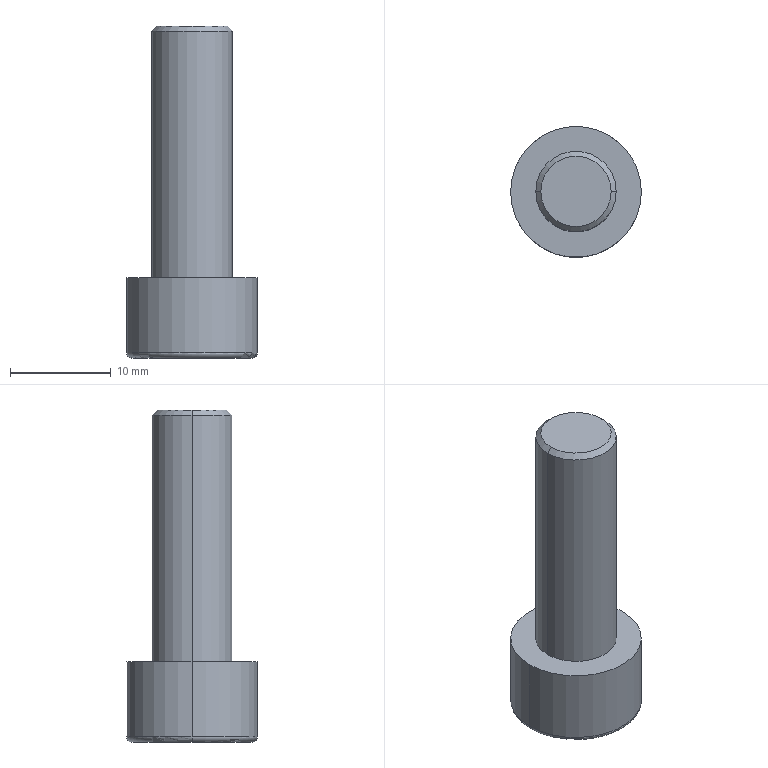Part | NX | features BREP 1 | 1 solid | 25 faces | box 13 x 13 x 33 mm | volume 2172 mm3 | plane 15 | cone 4 | cylinder 4 | torus 2 | commonest cylinder face diameters 8 x2 13 x2
STEP:
#1=CARTESIAN_POINT('',(0.,0.,5.732));
#2=VERTEX_POINT('',#1);
#3=CARTESIAN_POINT('',(-3.,0.,4.));
#4=VERTEX_POINT('',#3);
#5=CARTESIAN_POINT('',(-3.,0.,4.));
#6=DIRECTION('',(-0.866,0.,-0.5));
#7=VECTOR('',#6,1000.);
#8=LINE('',#5,#7);
#9=EDGE_CURVE('',#2,#4,#8,.T.);
#10=ORIENTED_EDGE('',*,*,#9,.F.);
#11=CARTESIAN_POINT('',(3.,0.,4.));
#12=VERTEX_POINT('',#11);
#13=CARTESIAN_POINT('',(3.,0.,4.));
#14=DIRECTION('',(0.866,0.,-0.5));
#15=VECTOR('',#14,1000.);
#16=LINE('',#13,#15);
#17=EDGE_CURVE('',#2,#12,#16,.T.);
#18=ORIENTED_EDGE('',*,*,#17,.T.);
#19=CARTESIAN_POINT('',(2.598,-1.5,4.));
#20=VERTEX_POINT('',#19);
#21=CARTESIAN_POINT('',(0.,0.,4.));
#22=DIRECTION('',(0.,0.,-1.));
#23=DIRECTION('',(-1.,0.,0.));
#24=AXIS2_PLACEMENT_3D('',#21,#22,#23);
#25=CIRCLE('',#24,3.);
#26=EDGE_CURVE('',#12,#20,#25,.T.);
#27=ORIENTED_EDGE('',*,*,#26,.T.);
#28=CARTESIAN_POINT('',(0.,-3.,4.));
#29=VERTEX_POINT('',#28);
#30=CARTESIAN_POINT('',(0.,0.,4.));
#31=DIRECTION('',(0.,0.,-1.));
#32=DIRECTION('',(-1.,0.,0.));
#33=AXIS2_PLACEMENT_3D('',#30,#31,#32);
#34=CIRCLE('',#33,3.);
#35=EDGE_CURVE('',#20,#29,#34,.T.);
#36=ORIENTED_EDGE('',*,*,#35,.T.);
#37=CARTESIAN_POINT('',(-2.598,-1.5,4.));
#38=VERTEX_POINT('',#37);
#39=CARTESIAN_POINT('',(0.,0.,4.));
#40=DIRECTION('',(0.,0.,-1.));
#41=DIRECTION('',(-1.,0.,0.));
#42=AXIS2_PLACEMENT_3D('',#39,#40,#41);
#43=CIRCLE('',#42,3.);
#44=EDGE_CURVE('',#29,#38,#43,.T.);
#45=ORIENTED_EDGE('',*,*,#44,.T.);
#46=CARTESIAN_POINT('',(0.,0.,4.));
#47=DIRECTION('',(0.,0.,-1.));
#48=DIRECTION('',(-1.,0.,0.));
#49=AXIS2_PLACEMENT_3D('',#46,#47,#48);
#50=CIRCLE('',#49,3.);
#51=EDGE_CURVE('',#38,#4,#50,.T.);
#52=ORIENTED_EDGE('',*,*,#51,.T.);
#53=EDGE_LOOP('',(#10,#18,#27,#36,#45,#52));
#54=FACE_BOUND('',#53,.T.);
#55=CARTESIAN_POINT('',(0.,0.,4.));
#56=DIRECTION('',(0.,0.,-1.));
#57=DIRECTION('',(-1.,0.,0.));
#58=AXIS2_PLACEMENT_3D('',#55,#56,#57);
#59=CONICAL_SURFACE('',#58,3.,1.047);
#60=ADVANCED_FACE('',(#54),#59,.F.);
#61=CARTESIAN_POINT('',(3.5,0.,33.));
#62=VERTEX_POINT('',#61);
#63=CARTESIAN_POINT('',(-3.5,0.,33.));
#64=VERTEX_POINT('',#63);
#65=CARTESIAN_POINT('',(0.,0.,33.));
#66=DIRECTION('',(0.,0.,1.));
#67=DIRECTION('',(1.,0.,0.));
#68=AXIS2_PLACEMENT_3D('',#65,#66,#67);
#69=CIRCLE('',#68,3.5);
#70=EDGE_CURVE('',#62,#64,#69,.T.);
#71=ORIENTED_EDGE('',*,*,#70,.F.);
#72=CARTESIAN_POINT('',(4.,0.,32.5));
#73=VERTEX_POINT('',#72);
#74=CARTESIAN_POINT('',(3.5,0.,33.));
#75=DIRECTION('',(0.7071,0.,-0.7071));
#76=VECTOR('',#75,1000.);
#77=LINE('',#74,#76);
#78=EDGE_CURVE('',#62,#73,#77,.T.);
#79=ORIENTED_EDGE('',*,*,#78,.T.);
#80=CARTESIAN_POINT('',(-4.,0.,32.5));
#81=VERTEX_POINT('',#80);
#82=CARTESIAN_POINT('',(0.,0.,32.5));
#83=DIRECTION('',(0.,0.,-1.));
#84=DIRECTION('',(1.,0.,0.));
#85=AXIS2_PLACEMENT_3D('',#82,#83,#84);
#86=CIRCLE('',#85,4.);
#87=EDGE_CURVE('',#81,#73,#86,.T.);
#88=ORIENTED_EDGE('',*,*,#87,.F.);
#89=CARTESIAN_POINT('',(-3.5,0.,33.));
#90=DIRECTION('',(-0.7071,0.,-0.7071));
#91=VECTOR('',#90,1000.);
#92=LINE('',#89,#91);
#93=EDGE_CURVE('',#64,#81,#92,.T.);
#94=ORIENTED_EDGE('',*,*,#93,.F.);
#95=EDGE_LOOP('',(#71,#79,#88,#94));
#96=FACE_BOUND('',#95,.T.);
#97=CARTESIAN_POINT('',(0.,0.,33.));
#98=DIRECTION('',(0.,0.,-1.));
#99=DIRECTION('',(-1.,0.,0.));
#100=AXIS2_PLACEMENT_3D('',#97,#98,#99);
#101=CONICAL_SURFACE('',#100,3.5,0.7854);
#102=ADVANCED_FACE('',(#96),#101,.T.);
#103=CARTESIAN_POINT('',(-6.,0.,0.));
#104=VERTEX_POINT('',#103);
#105=CARTESIAN_POINT('',(6.,0.,0.));
#106=VERTEX_POINT('',#105);
#107=CARTESIAN_POINT('',(0.,0.,0.));
#108=DIRECTION('',(0.,0.,-1.));
#109=DIRECTION('',(1.,0.,0.));
#110=AXIS2_PLACEMENT_3D('',#107,#108,#109);
#111=CIRCLE('',#110,6.);
#112=EDGE_CURVE('',#104,#106,#111,.T.);
#113=ORIENTED_EDGE('',*,*,#112,.F.);
#114=CARTESIAN_POINT('',(-6.5,0.,0.5));
#115=VERTEX_POINT('',#114);
#116=CARTESIAN_POINT('',(-6.,0.,0.5));
#117=DIRECTION('',(0.,1.,0.));
#118=DIRECTION('',(-1.,0.,0.));
#119=AXIS2_PLACEMENT_3D('',#116,#117,#118);
#120=CIRCLE('',#119,0.5);
#121=EDGE_CURVE('',#115,#104,#120,.F.);
#122=ORIENTED_EDGE('',*,*,#121,.F.);
#123=CARTESIAN_POINT('',(6.5,0.,0.5));
#124=VERTEX_POINT('',#123);
#125=CARTESIAN_POINT('',(0.,0.,0.5));
#126=DIRECTION('',(0.,0.,1.));
#127=DIRECTION('',(1.,0.,0.));
#128=AXIS2_PLACEMENT_3D('',#125,#126,#127);
#129=CIRCLE('',#128,6.5);
#130=EDGE_CURVE('',#124,#115,#129,.T.);
#131=ORIENTED_EDGE('',*,*,#130,.F.);
#132=CARTESIAN_POINT('',(6.,0.,0.5));
#133=DIRECTION('',(0.,-1.,0.));
#134=DIRECTION('',(0.,0.,-1.));
#135=AXIS2_PLACEMENT_3D('',#132,#133,#134);
#136=CIRCLE('',#135,0.5);
#137=EDGE_CURVE('',#124,#106,#136,.F.);
#138=ORIENTED_EDGE('',*,*,#137,.T.);
#139=EDGE_LOOP('',(#113,#122,#131,#138));
#140=FACE_BOUND('',#139,.T.);
#141=CARTESIAN_POINT('',(0.,0.,0.5));
#142=DIRECTION('',(0.,0.,1.));
#143=DIRECTION('',(1.,0.,0.));
#144=AXIS2_PLACEMENT_3D('',#141,#142,#143);
#145=TOROIDAL_SURFACE('',#144,6.,0.5);
#146=ADVANCED_FACE('',(#140),#145,.T.);
#147=ORIENTED_EDGE('',*,*,#87,.T.);
#148=CARTESIAN_POINT('',(4.,0.,8.));
#149=VERTEX_POINT('',#148);
#150=CARTESIAN_POINT('',(4.,0.,33.));
#151=DIRECTION('',(0.,0.,-1.));
#152=VECTOR('',#151,1000.);
#153=LINE('',#150,#152);
#154=EDGE_CURVE('',#73,#149,#153,.T.);
#155=ORIENTED_EDGE('',*,*,#154,.T.);
#156=CARTESIAN_POINT('',(-4.,0.,8.));
#157=VERTEX_POINT('',#156);
#158=CARTESIAN_POINT('',(0.,0.,8.));
#159=DIRECTION('',(0.,0.,1.));
#160=DIRECTION('',(1.,0.,0.));
#161=AXIS2_PLACEMENT_3D('',#158,#159,#160);
#162=CIRCLE('',#161,4.);
#163=EDGE_CURVE('',#149,#157,#162,.T.);
#164=ORIENTED_EDGE('',*,*,#163,.T.);
#165=CARTESIAN_POINT('',(-4.,0.,33.));
#166=DIRECTION('',(0.,0.,-1.));
#167=VECTOR('',#166,1000.);
#168=LINE('',#165,#167);
#169=EDGE_CURVE('',#81,#157,#168,.T.);
#170=ORIENTED_EDGE('',*,*,#169,.F.);
#171=EDGE_LOOP('',(#147,#155,#164,#170));
#172=FACE_BOUND('',#171,.T.);
#173=CARTESIAN_POINT('',(0.,0.,33.));
#174=DIRECTION('',(0.,0.,-1.));
#175=DIRECTION('',(-1.,0.,0.));
#176=AXIS2_PLACEMENT_3D('',#173,#174,#175);
#177=CYLINDRICAL_SURFACE('',#176,4.);
#178=ADVANCED_FACE('',(#172),#177,.T.);
#179=CARTESIAN_POINT('',(6.5,0.,8.));
#180=VERTEX_POINT('',#179);
#181=CARTESIAN_POINT('',(-6.5,0.,8.));
#182=VERTEX_POINT('',#181);
#183=CARTESIAN_POINT('',(0.,0.,8.));
#184=DIRECTION('',(0.,0.,1.));
#185=DIRECTION('',(1.,0.,0.));
#186=AXIS2_PLACEMENT_3D('',#183,#184,#185);
#187=CIRCLE('',#186,6.5);
#188=EDGE_CURVE('',#180,#182,#187,.T.);
#189=ORIENTED_EDGE('',*,*,#188,.F.);
#190=CARTESIAN_POINT('',(6.5,0.,8.));
#191=DIRECTION('',(0.,0.,-1.));
#192=VECTOR('',#191,1000.);
#193=LINE('',#190,#192);
#194=EDGE_CURVE('',#180,#124,#193,.T.);
#195=ORIENTED_EDGE('',*,*,#194,.T.);
#196=ORIENTED_EDGE('',*,*,#130,.T.);
#197=CARTESIAN_POINT('',(-6.5,0.,8.));
#198=DIRECTION('',(0.,0.,-1.));
#199=VECTOR('',#198,1000.);
#200=LINE('',#197,#199);
#201=EDGE_CURVE('',#182,#115,#200,.T.);
#202=ORIENTED_EDGE('',*,*,#201,.F.);
#203=EDGE_LOOP('',(#189,#195,#196,#202));
#204=FACE_BOUND('',#203,.T.);
#205=CARTESIAN_POINT('',(0.,0.,8.));
#206=DIRECTION('',(0.,0.,-1.));
#207=DIRECTION('',(-1.,0.,0.));
#208=AXIS2_PLACEMENT_3D('',#205,#206,#207);
#209=CYLINDRICAL_SURFACE('',#208,6.5);
#210=ADVANCED_FACE('',(#204),#209,.T.);
#211=CARTESIAN_POINT('',(-2.598,1.5,4.));
#212=VERTEX_POINT('',#211);
#213=CARTESIAN_POINT('',(0.,3.,4.));
#214=VERTEX_POINT('',#213);
#215=CARTESIAN_POINT('',(0.,0.,4.));
#216=DIRECTION('',(0.,0.,-1.));
#217=DIRECTION('',(-1.,0.,0.));
#218=AXIS2_PLACEMENT_3D('',#215,#216,#217);
#219=CIRCLE('',#218,3.);
#220=EDGE_CURVE('',#212,#214,#219,.T.);
#221=ORIENTED_EDGE('',*,*,#220,.F.);
#222=CARTESIAN_POINT('',(-1.732,3.,4.));
#223=VERTEX_POINT('',#222);
#224=CARTESIAN_POINT('',(-3.464,0.,4.));
#225=DIRECTION('',(0.5,0.866,0.));
#226=VECTOR('',#225,1000.);
#227=LINE('',#224,#226);
#228=EDGE_CURVE('',#212,#223,#227,.T.);
#229=ORIENTED_EDGE('',*,*,#228,.T.);
#230=CARTESIAN_POINT('',(-1.732,3.,4.));
#231=DIRECTION('',(1.,0.,0.));
#232=VECTOR('',#231,1000.);
#233=LINE('',#230,#232);
#234=EDGE_CURVE('',#223,#214,#233,.T.);
#235=ORIENTED_EDGE('',*,*,#234,.T.);
#236=EDGE_LOOP('',(#221,#229,#235));
#237=FACE_BOUND('',#236,.T.);
#238=CARTESIAN_POINT('',(0.,0.,4.));
#239=DIRECTION('',(0.,0.,-1.));
#240=DIRECTION('',(0.,-1.,0.));
#241=AXIS2_PLACEMENT_3D('',#238,#239,#240);
#242=PLANE('',#241);
#243=ADVANCED_FACE('',(#237),#242,.T.);
#244=CARTESIAN_POINT('',(2.598,1.5,4.));
#245=VERTEX_POINT('',#244);
#246=CARTESIAN_POINT('',(0.,0.,4.));
#247=DIRECTION('',(0.,0.,-1.));
#248=DIRECTION('',(-1.,0.,0.));
#249=AXIS2_PLACEMENT_3D('',#246,#247,#248);
#250=CIRCLE('',#249,3.);
#251=EDGE_CURVE('',#214,#245,#250,.T.);
#252=ORIENTED_EDGE('',*,*,#251,.F.);
#253=CARTESIAN_POINT('',(1.732,3.,4.));
#254=VERTEX_POINT('',#253);
#255=CARTESIAN_POINT('',(-1.732,3.,4.));
#256=DIRECTION('',(1.,0.,0.));
#257=VECTOR('',#256,1000.);
#258=LINE('',#255,#257);
#259=EDGE_CURVE('',#214,#254,#258,.T.);
#260=ORIENTED_EDGE('',*,*,#259,.T.);
#261=CARTESIAN_POINT('',(1.732,3.,4.));
#262=DIRECTION('',(0.5,-0.866,0.));
#263=VECTOR('',#262,1000.);
#264=LINE('',#261,#263);
#265=EDGE_CURVE('',#254,#245,#264,.T.);
#266=ORIENTED_EDGE('',*,*,#265,.T.);
#267=EDGE_LOOP('',(#252,#260,#266));
#268=FACE_BOUND('',#267,.T.);
#269=CARTESIAN_POINT('',(0.,0.,4.));
#270=DIRECTION('',(0.,0.,-1.));
#271=DIRECTION('',(0.,-1.,0.));
#272=AXIS2_PLACEMENT_3D('',#269,#270,#271);
#273=PLANE('',#272);
#274=ADVANCED_FACE('',(#268),#273,.T.);
#275=CARTESIAN_POINT('',(0.,0.,4.));
#276=DIRECTION('',(0.,0.,-1.));
#277=DIRECTION('',(-1.,0.,0.));
#278=AXIS2_PLACEMENT_3D('',#275,#276,#277);
#279=CIRCLE('',#278,3.);
#280=EDGE_CURVE('',#245,#12,#279,.T.);
#281=ORIENTED_EDGE('',*,*,#280,.F.);
#282=CARTESIAN_POINT('',(3.464,0.,4.));
#283=VERTEX_POINT('',#282);
#284=CARTESIAN_POINT('',(1.732,3.,4.));
#285=DIRECTION('',(0.5,-0.866,0.));
#286=VECTOR('',#285,1000.);
#287=LINE('',#284,#286);
#288=EDGE_CURVE('',#245,#283,#287,.T.);
#289=ORIENTED_EDGE('',*,*,#288,.T.);
#290=CARTESIAN_POINT('',(3.464,0.,4.));
#291=DIRECTION('',(-0.5,-0.866,0.));
#292=VECTOR('',#291,1000.);
#293=LINE('',#290,#292);
#294=EDGE_CURVE('',#283,#20,#293,.T.);
#295=ORIENTED_EDGE('',*,*,#294,.T.);
#296=ORIENTED_EDGE('',*,*,#26,.F.);
#297=EDGE_LOOP('',(#281,#289,#295,#296));
#298=FACE_BOUND('',#297,.T.);
#299=CARTESIAN_POINT('',(0.,0.,4.));
#300=DIRECTION('',(0.,0.,-1.));
#301=DIRECTION('',(0.,-1.,0.));
#302=AXIS2_PLACEMENT_3D('',#299,#300,#301);
#303=PLANE('',#302);
#304=ADVANCED_FACE('',(#298),#303,.T.);
#305=ORIENTED_EDGE('',*,*,#35,.F.);
#306=CARTESIAN_POINT('',(1.732,-3.,4.));
#307=VERTEX_POINT('',#306);
#308=CARTESIAN_POINT('',(3.464,0.,4.));
#309=DIRECTION('',(-0.5,-0.866,0.));
#310=VECTOR('',#309,1000.);
#311=LINE('',#308,#310);
#312=EDGE_CURVE('',#20,#307,#311,.T.);
#313=ORIENTED_EDGE('',*,*,#312,.T.);
#314=CARTESIAN_POINT('',(1.732,-3.,4.));
#315=DIRECTION('',(-1.,0.,0.));
#316=VECTOR('',#315,1000.);
#317=LINE('',#314,#316);
#318=EDGE_CURVE('',#307,#29,#317,.T.);
#319=ORIENTED_EDGE('',*,*,#318,.T.);
#320=EDGE_LOOP('',(#305,#313,#319));
#321=FACE_BOUND('',#320,.T.);
#322=CARTESIAN_POINT('',(0.,0.,4.));
#323=DIRECTION('',(0.,0.,-1.));
#324=DIRECTION('',(0.,-1.,0.));
#325=AXIS2_PLACEMENT_3D('',#322,#323,#324);
#326=PLANE('',#325);
#327=ADVANCED_FACE('',(#321),#326,.T.);
#328=ORIENTED_EDGE('',*,*,#44,.F.);
#329=CARTESIAN_POINT('',(-1.732,-3.,4.));
#330=VERTEX_POINT('',#329);
#331=CARTESIAN_POINT('',(1.732,-3.,4.));
#332=DIRECTION('',(-1.,0.,0.));
#333=VECTOR('',#332,1000.);
#334=LINE('',#331,#333);
#335=EDGE_CURVE('',#29,#330,#334,.T.);
#336=ORIENTED_EDGE('',*,*,#335,.T.);
#337=CARTESIAN_POINT('',(-1.732,-3.,4.));
#338=DIRECTION('',(-0.5,0.866,0.));
#339=VECTOR('',#338,1000.);
#340=LINE('',#337,#339);
#341=EDGE_CURVE('',#330,#38,#340,.T.);
#342=ORIENTED_EDGE('',*,*,#341,.T.);
#343=EDGE_LOOP('',(#328,#336,#342));
#344=FACE_BOUND('',#343,.T.);
#345=CARTESIAN_POINT('',(0.,0.,4.));
#346=DIRECTION('',(0.,0.,-1.));
#347=DIRECTION('',(0.,-1.,0.));
#348=AXIS2_PLACEMENT_3D('',#345,#346,#347);
#349=PLANE('',#348);
#350=ADVANCED_FACE('',(#344),#349,.T.);
#351=CARTESIAN_POINT('',(0.,0.,8.));
#352=DIRECTION('',(0.,0.,1.));
#353=DIRECTION('',(1.,0.,0.));
#354=AXIS2_PLACEMENT_3D('',#351,#352,#353);
#355=CIRCLE('',#354,6.5);
#356=EDGE_CURVE('',#182,#180,#355,.T.);
#357=ORIENTED_EDGE('',*,*,#356,.T.);
#358=ORIENTED_EDGE('',*,*,#188,.T.);
#359=EDGE_LOOP('',(#357,#358));
#360=FACE_BOUND('',#359,.T.);
#361=CARTESIAN_POINT('',(0.,0.,8.));
#362=DIRECTION('',(0.,0.,1.));
#363=DIRECTION('',(1.,0.,0.));
#364=AXIS2_PLACEMENT_3D('',#361,#362,#363);
#365=CIRCLE('',#364,4.);
#366=EDGE_CURVE('',#157,#149,#365,.T.);
#367=ORIENTED_EDGE('',*,*,#366,.F.);
#368=ORIENTED_EDGE('',*,*,#163,.F.);
#369=EDGE_LOOP('',(#367,#368));
#370=FACE_BOUND('',#369,.T.);
#371=CARTESIAN_POINT('',(0.,0.,8.));
#372=DIRECTION('',(0.,0.,1.));
#373=DIRECTION('',(1.,0.,0.));
#374=AXIS2_PLACEMENT_3D('',#371,#372,#373);
#375=PLANE('',#374);
#376=ADVANCED_FACE('',(#360,#370),#375,.T.);
#377=ORIENTED_EDGE('',*,*,#194,.F.);
#378=ORIENTED_EDGE('',*,*,#356,.F.);
#379=ORIENTED_EDGE('',*,*,#201,.T.);
#380=CARTESIAN_POINT('',(0.,0.,0.5));
#381=DIRECTION('',(0.,0.,1.));
#382=DIRECTION('',(1.,0.,0.));
#383=AXIS2_PLACEMENT_3D('',#380,#381,#382);
#384=CIRCLE('',#383,6.5);
#385=EDGE_CURVE('',#115,#124,#384,.T.);
#386=ORIENTED_EDGE('',*,*,#385,.T.);
#387=EDGE_LOOP('',(#377,#378,#379,#386));
#388=FACE_BOUND('',#387,.T.);
#389=CARTESIAN_POINT('',(0.,0.,8.));
#390=DIRECTION('',(0.,0.,-1.));
#391=DIRECTION('',(-1.,0.,0.));
#392=AXIS2_PLACEMENT_3D('',#389,#390,#391);
#393=CYLINDRICAL_SURFACE('',#392,6.5);
#394=ADVANCED_FACE('',(#388),#393,.T.);
#395=CARTESIAN_POINT('',(0.,0.,0.));
#396=DIRECTION('',(0.,0.,-1.));
#397=DIRECTION('',(1.,0.,0.));
#398=AXIS2_PLACEMENT_3D('',#395,#396,#397);
#399=CIRCLE('',#398,6.);
#400=EDGE_CURVE('',#106,#104,#399,.T.);
#401=ORIENTED_EDGE('',*,*,#400,.T.);
#402=ORIENTED_EDGE('',*,*,#112,.T.);
#403=EDGE_LOOP('',(#401,#402));
#404=FACE_BOUND('',#403,.T.);
#405=CARTESIAN_POINT('',(-1.732,3.,0.));
#406=VERTEX_POINT('',#405);
#407=CARTESIAN_POINT('',(1.732,3.,0.));
#408=VERTEX_POINT('',#407);
#409=CARTESIAN_POINT('',(-1.732,3.,0.));
#410=DIRECTION('',(1.,0.,0.));
#411=VECTOR('',#410,1000.);
#412=LINE('',#409,#411);
#413=EDGE_CURVE('',#406,#408,#412,.T.);
#414=ORIENTED_EDGE('',*,*,#413,.F.);
#415=CARTESIAN_POINT('',(-3.464,0.,0.));
#416=VERTEX_POINT('',#415);
#417=CARTESIAN_POINT('',(-3.464,0.,0.));
#418=DIRECTION('',(0.5,0.866,0.));
#419=VECTOR('',#418,1000.);
#420=LINE('',#417,#419);
#421=EDGE_CURVE('',#416,#406,#420,.T.);
#422=ORIENTED_EDGE('',*,*,#421,.F.);
#423=CARTESIAN_POINT('',(-1.732,-3.,0.));
#424=VERTEX_POINT('',#423);
#425=CARTESIAN_POINT('',(-1.732,-3.,0.));
#426=DIRECTION('',(-0.5,0.866,0.));
#427=VECTOR('',#426,1000.);
#428=LINE('',#425,#427);
#429=EDGE_CURVE('',#424,#416,#428,.T.);
#430=ORIENTED_EDGE('',*,*,#429,.F.);
#431=CARTESIAN_POINT('',(1.732,-3.,0.));
#432=VERTEX_POINT('',#431);
#433=CARTESIAN_POINT('',(1.732,-3.,0.));
#434=DIRECTION('',(-1.,0.,0.));
#435=VECTOR('',#434,1000.);
#436=LINE('',#433,#435);
#437=EDGE_CURVE('',#432,#424,#436,.T.);
#438=ORIENTED_EDGE('',*,*,#437,.F.);
#439=CARTESIAN_POINT('',(3.464,0.,0.));
#440=VERTEX_POINT('',#439);
#441=CARTESIAN_POINT('',(3.464,0.,0.));
#442=DIRECTION('',(-0.5,-0.866,0.));
#443=VECTOR('',#442,1000.);
#444=LINE('',#441,#443);
#445=EDGE_CURVE('',#440,#432,#444,.T.);
#446=ORIENTED_EDGE('',*,*,#445,.F.);
#447=CARTESIAN_POINT('',(1.732,3.,0.));
#448=DIRECTION('',(0.5,-0.866,0.));
#449=VECTOR('',#448,1000.);
#450=LINE('',#447,#449);
#451=EDGE_CURVE('',#408,#440,#450,.T.);
#452=ORIENTED_EDGE('',*,*,#451,.F.);
#453=EDGE_LOOP('',(#414,#422,#430,#438,#446,#452));
#454=FACE_BOUND('',#453,.T.);
#455=CARTESIAN_POINT('',(0.,0.,0.));
#456=DIRECTION('',(0.,0.,1.));
#457=DIRECTION('',(1.,0.,0.));
#458=AXIS2_PLACEMENT_3D('',#455,#456,#457);
#459=PLANE('',#458);
#460=ADVANCED_FACE('',(#404,#454),#459,.F.);
#461=ORIENTED_EDGE('',*,*,#154,.F.);
#462=CARTESIAN_POINT('',(0.,0.,32.5));
#463=DIRECTION('',(0.,0.,-1.));
#464=DIRECTION('',(1.,0.,0.));
#465=AXIS2_PLACEMENT_3D('',#462,#463,#464);
#466=CIRCLE('',#465,4.);
#467=EDGE_CURVE('',#73,#81,#466,.T.);
#468=ORIENTED_EDGE('',*,*,#467,.T.);
#469=ORIENTED_EDGE('',*,*,#169,.T.);
#470=ORIENTED_EDGE('',*,*,#366,.T.);
#471=EDGE_LOOP('',(#461,#468,#469,#470));
#472=FACE_BOUND('',#471,.T.);
#473=CARTESIAN_POINT('',(0.,0.,33.));
#474=DIRECTION('',(0.,0.,-1.));
#475=DIRECTION('',(-1.,0.,0.));
#476=AXIS2_PLACEMENT_3D('',#473,#474,#475);
#477=CYLINDRICAL_SURFACE('',#476,4.);
#478=ADVANCED_FACE('',(#472),#477,.T.);
#479=CARTESIAN_POINT('',(0.,0.,33.));
#480=DIRECTION('',(0.,0.,1.));
#481=DIRECTION('',(1.,0.,0.));
#482=AXIS2_PLACEMENT_3D('',#479,#480,#481);
#483=CIRCLE('',#482,3.5);
#484=EDGE_CURVE('',#64,#62,#483,.T.);
#485=ORIENTED_EDGE('',*,*,#484,.T.);
#486=ORIENTED_EDGE('',*,*,#70,.T.);
#487=EDGE_LOOP('',(#485,#486));
#488=FACE_BOUND('',#487,.T.);
#489=CARTESIAN_POINT('',(0.,0.,33.));
#490=DIRECTION('',(0.,0.,1.));
#491=DIRECTION('',(1.,0.,0.));
#492=AXIS2_PLACEMENT_3D('',#489,#490,#491);
#493=PLANE('',#492);
#494=ADVANCED_FACE('',(#488),#493,.T.);
#495=ORIENTED_EDGE('',*,*,#121,.T.);
#496=ORIENTED_EDGE('',*,*,#400,.F.);
#497=ORIENTED_EDGE('',*,*,#137,.F.);
#498=ORIENTED_EDGE('',*,*,#385,.F.);
#499=EDGE_LOOP('',(#495,#496,#497,#498));
#500=FACE_BOUND('',#499,.T.);
#501=CARTESIAN_POINT('',(0.,0.,0.5));
#502=DIRECTION('',(0.,0.,1.));
#503=DIRECTION('',(1.,0.,0.));
#504=AXIS2_PLACEMENT_3D('',#501,#502,#503);
#505=TOROIDAL_SURFACE('',#504,6.,0.5);
#506=ADVANCED_FACE('',(#500),#505,.T.);
#507=ORIENTED_EDGE('',*,*,#78,.F.);
#508=ORIENTED_EDGE('',*,*,#484,.F.);
#509=ORIENTED_EDGE('',*,*,#93,.T.);
#510=ORIENTED_EDGE('',*,*,#467,.F.);
#511=EDGE_LOOP('',(#507,#508,#509,#510));
#512=FACE_BOUND('',#511,.T.);
#513=CARTESIAN_POINT('',(0.,0.,33.));
#514=DIRECTION('',(0.,0.,-1.));
#515=DIRECTION('',(-1.,0.,0.));
#516=AXIS2_PLACEMENT_3D('',#513,#514,#515);
#517=CONICAL_SURFACE('',#516,3.5,0.7854);
#518=ADVANCED_FACE('',(#512),#517,.T.);
#519=ORIENTED_EDGE('',*,*,#421,.T.);
#520=CARTESIAN_POINT('',(-1.732,3.,4.));
#521=DIRECTION('',(0.,0.,-1.));
#522=VECTOR('',#521,1000.);
#523=LINE('',#520,#522);
#524=EDGE_CURVE('',#223,#406,#523,.T.);
#525=ORIENTED_EDGE('',*,*,#524,.F.);
#526=ORIENTED_EDGE('',*,*,#228,.F.);
#527=CARTESIAN_POINT('',(-3.464,0.,4.));
#528=VERTEX_POINT('',#527);
#529=CARTESIAN_POINT('',(-3.464,0.,4.));
#530=DIRECTION('',(0.5,0.866,0.));
#531=VECTOR('',#530,1000.);
#532=LINE('',#529,#531);
#533=EDGE_CURVE('',#528,#212,#532,.T.);
#534=ORIENTED_EDGE('',*,*,#533,.F.);
#535=CARTESIAN_POINT('',(-3.464,0.,4.));
#536=DIRECTION('',(0.,0.,-1.));
#537=VECTOR('',#536,1000.);
#538=LINE('',#535,#537);
#539=EDGE_CURVE('',#528,#416,#538,.T.);
#540=ORIENTED_EDGE('',*,*,#539,.T.);
#541=EDGE_LOOP('',(#519,#525,#526,#534,#540));
#542=FACE_BOUND('',#541,.T.);
#543=CARTESIAN_POINT('',(-3.464,0.,4.));
#544=DIRECTION('',(-0.866,0.5,0.));
#545=DIRECTION('',(0.,0.,1.));
#546=AXIS2_PLACEMENT_3D('',#543,#544,#545);
#547=PLANE('',#546);
#548=ADVANCED_FACE('',(#542),#547,.F.);
#549=ORIENTED_EDGE('',*,*,#429,.T.);
#550=ORIENTED_EDGE('',*,*,#539,.F.);
#551=CARTESIAN_POINT('',(-1.732,-3.,4.));
#552=DIRECTION('',(-0.5,0.866,0.));
#553=VECTOR('',#552,1000.);
#554=LINE('',#551,#553);
#555=EDGE_CURVE('',#38,#528,#554,.T.);
#556=ORIENTED_EDGE('',*,*,#555,.F.);
#557=ORIENTED_EDGE('',*,*,#341,.F.);
#558=CARTESIAN_POINT('',(-1.732,-3.,4.));
#559=DIRECTION('',(0.,0.,-1.));
#560=VECTOR('',#559,1000.);
#561=LINE('',#558,#560);
#562=EDGE_CURVE('',#330,#424,#561,.T.);
#563=ORIENTED_EDGE('',*,*,#562,.T.);
#564=EDGE_LOOP('',(#549,#550,#556,#557,#563));
#565=FACE_BOUND('',#564,.T.);
#566=CARTESIAN_POINT('',(-1.732,-3.,4.));
#567=DIRECTION('',(-0.866,-0.5,0.));
#568=DIRECTION('',(-0.5,0.866,0.));
#569=AXIS2_PLACEMENT_3D('',#566,#567,#568);
#570=PLANE('',#569);
#571=ADVANCED_FACE('',(#565),#570,.F.);
#572=ORIENTED_EDGE('',*,*,#437,.T.);
#573=ORIENTED_EDGE('',*,*,#562,.F.);
#574=ORIENTED_EDGE('',*,*,#335,.F.);
#575=ORIENTED_EDGE('',*,*,#318,.F.);
#576=CARTESIAN_POINT('',(1.732,-3.,4.));
#577=DIRECTION('',(0.,0.,-1.));
#578=VECTOR('',#577,1000.);
#579=LINE('',#576,#578);
#580=EDGE_CURVE('',#307,#432,#579,.T.);
#581=ORIENTED_EDGE('',*,*,#580,.T.);
#582=EDGE_LOOP('',(#572,#573,#574,#575,#581));
#583=FACE_BOUND('',#582,.T.);
#584=CARTESIAN_POINT('',(1.732,-3.,4.));
#585=DIRECTION('',(0.,-1.,0.));
#586=DIRECTION('',(0.,0.,-1.));
#587=AXIS2_PLACEMENT_3D('',#584,#585,#586);
#588=PLANE('',#587);
#589=ADVANCED_FACE('',(#583),#588,.F.);
#590=ORIENTED_EDGE('',*,*,#445,.T.);
#591=ORIENTED_EDGE('',*,*,#580,.F.);
#592=ORIENTED_EDGE('',*,*,#312,.F.);
#593=ORIENTED_EDGE('',*,*,#294,.F.);
#594=CARTESIAN_POINT('',(3.464,0.,4.));
#595=DIRECTION('',(0.,0.,-1.));
#596=VECTOR('',#595,1000.);
#597=LINE('',#594,#596);
#598=EDGE_CURVE('',#283,#440,#597,.T.);
#599=ORIENTED_EDGE('',*,*,#598,.T.);
#600=EDGE_LOOP('',(#590,#591,#592,#593,#599));
#601=FACE_BOUND('',#600,.T.);
#602=CARTESIAN_POINT('',(3.464,0.,4.));
#603=DIRECTION('',(0.866,-0.5,0.));
#604=DIRECTION('',(0.,0.,-1.));
#605=AXIS2_PLACEMENT_3D('',#602,#603,#604);
#606=PLANE('',#605);
#607=ADVANCED_FACE('',(#601),#606,.F.);
#608=ORIENTED_EDGE('',*,*,#451,.T.);
#609=ORIENTED_EDGE('',*,*,#598,.F.);
#610=ORIENTED_EDGE('',*,*,#288,.F.);
#611=ORIENTED_EDGE('',*,*,#265,.F.);
#612=CARTESIAN_POINT('',(1.732,3.,4.));
#613=DIRECTION('',(0.,0.,-1.));
#614=VECTOR('',#613,1000.);
#615=LINE('',#612,#614);
#616=EDGE_CURVE('',#254,#408,#615,.T.);
#617=ORIENTED_EDGE('',*,*,#616,.T.);
#618=EDGE_LOOP('',(#608,#609,#610,#611,#617));
#619=FACE_BOUND('',#618,.T.);
#620=CARTESIAN_POINT('',(1.732,3.,4.));
#621=DIRECTION('',(0.866,0.5,0.));
#622=DIRECTION('',(0.,0.,-1.));
#623=AXIS2_PLACEMENT_3D('',#620,#621,#622);
#624=PLANE('',#623);
#625=ADVANCED_FACE('',(#619),#624,.F.);
#626=ORIENTED_EDGE('',*,*,#413,.T.);
#627=ORIENTED_EDGE('',*,*,#616,.F.);
#628=ORIENTED_EDGE('',*,*,#259,.F.);
#629=ORIENTED_EDGE('',*,*,#234,.F.);
#630=ORIENTED_EDGE('',*,*,#524,.T.);
#631=EDGE_LOOP('',(#626,#627,#628,#629,#630));
#632=FACE_BOUND('',#631,.T.);
#633=CARTESIAN_POINT('',(-1.732,3.,4.));
#634=DIRECTION('',(0.,1.,0.));
#635=DIRECTION('',(1.,0.,0.));
#636=AXIS2_PLACEMENT_3D('',#633,#634,#635);
#637=PLANE('',#636);
#638=ADVANCED_FACE('',(#632),#637,.F.);
#639=ORIENTED_EDGE('',*,*,#51,.F.);
#640=ORIENTED_EDGE('',*,*,#555,.T.);
#641=ORIENTED_EDGE('',*,*,#533,.T.);
#642=CARTESIAN_POINT('',(0.,0.,4.));
#643=DIRECTION('',(0.,0.,-1.));
#644=DIRECTION('',(-1.,0.,0.));
#645=AXIS2_PLACEMENT_3D('',#642,#643,#644);
#646=CIRCLE('',#645,3.);
#647=EDGE_CURVE('',#4,#212,#646,.T.);
#648=ORIENTED_EDGE('',*,*,#647,.F.);
#649=EDGE_LOOP('',(#639,#640,#641,#648));
#650=FACE_BOUND('',#649,.T.);
#651=CARTESIAN_POINT('',(0.,0.,4.));
#652=DIRECTION('',(0.,0.,-1.));
#653=DIRECTION('',(0.,-1.,0.));
#654=AXIS2_PLACEMENT_3D('',#651,#652,#653);
#655=PLANE('',#654);
#656=ADVANCED_FACE('',(#650),#655,.T.);
#657=ORIENTED_EDGE('',*,*,#17,.F.);
#658=ORIENTED_EDGE('',*,*,#9,.T.);
#659=ORIENTED_EDGE('',*,*,#647,.T.);
#660=ORIENTED_EDGE('',*,*,#220,.T.);
#661=ORIENTED_EDGE('',*,*,#251,.T.);
#662=ORIENTED_EDGE('',*,*,#280,.T.);
#663=EDGE_LOOP('',(#657,#658,#659,#660,#661,#662));
#664=FACE_BOUND('',#663,.T.);
#665=CARTESIAN_POINT('',(0.,0.,4.));
#666=DIRECTION('',(0.,0.,-1.));
#667=DIRECTION('',(-1.,0.,0.));
#668=AXIS2_PLACEMENT_3D('',#665,#666,#667);
#669=CONICAL_SURFACE('',#668,3.,1.047);
#670=ADVANCED_FACE('',(#664),#669,.F.);
#671=CLOSED_SHELL('',(#60,#102,#146,#178,#210,#243,#274,#304,#327,#350,#376,#394,#460,#478,#494,#506,#518,#548,#571,#589,#607,#625,#638,#656,#670));
#672=MANIFOLD_SOLID_BREP('',#671);
#673=(LENGTH_UNIT()NAMED_UNIT(*)SI_UNIT(.MILLI.,.METRE.));
#674=UNCERTAINTY_MEASURE_WITH_UNIT(LENGTH_MEASURE(0.00001),#673,'','');
#675=(NAMED_UNIT(*)PLANE_ANGLE_UNIT()SI_UNIT($,.RADIAN.));
#676=(NAMED_UNIT(*)SI_UNIT($,.STERADIAN.)SOLID_ANGLE_UNIT());
#677=(GEOMETRIC_REPRESENTATION_CONTEXT(3)GLOBAL_UNCERTAINTY_ASSIGNED_CONTEXT((#674))GLOBAL_UNIT_ASSIGNED_CONTEXT((#673,#675,#676))REPRESENTATION_CONTEXT('',''));
#678=ADVANCED_BREP_SHAPE_REPRESENTATION('',(#672),#677);